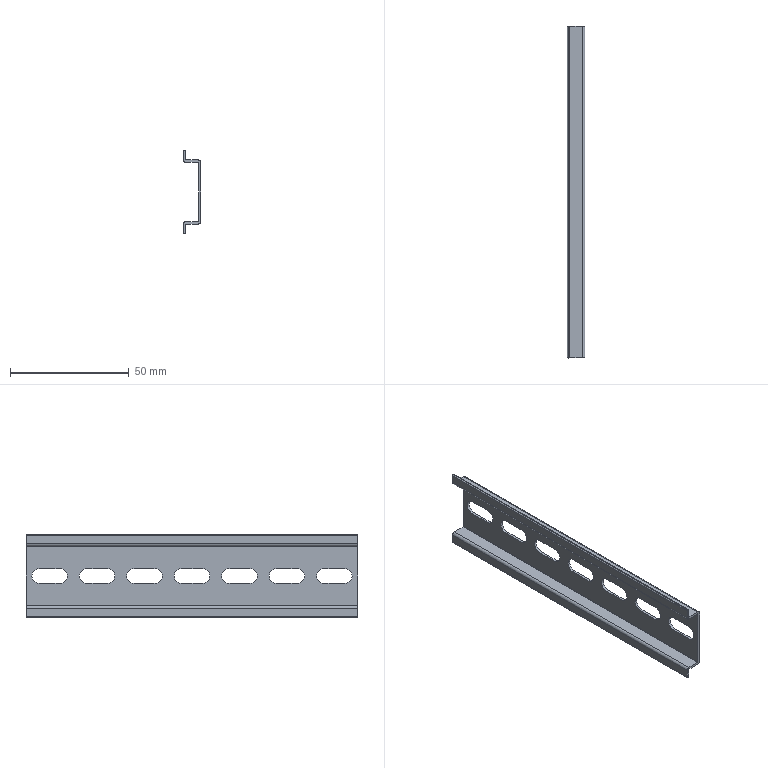Part | STEP file | 00 | 1 solid | 61 faces | box 7.5 x 140 x 35 mm | volume 5963 mm3 | cylinder 33 | plane 28 | commonest cylinder face diameters 6.2 x21 0.2 x4 0.8 x4 2.2 x4